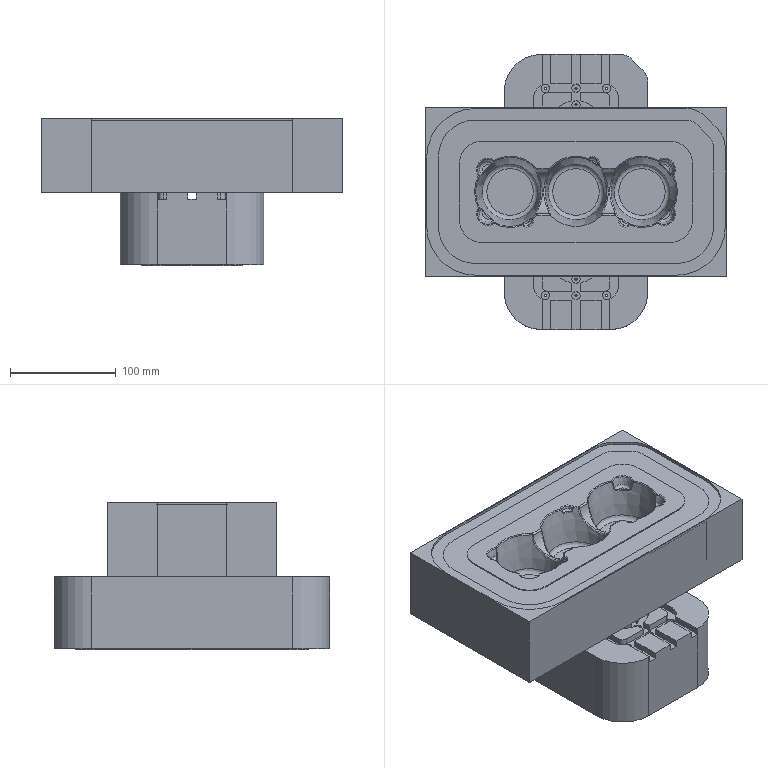NC program | NX | posted with a generic post | part box 284.317 x 260.317 x 139.5 mm
Lines 1 to 931 of 226982:
N10 G17 G21 G94 G90
(B1 , TOOL : D16R0.8)
N12 T00 M6
N14 G53
N16 G17 G0 G90 X-27.032 Y70.7 S7000 M3 M8
N18 G43 Z220.5 H0
N20 Z71.5
N22 G94 G1 X0. Z70.083 F4500.
N24 X103.946
N26 G2 X116.548 Y65.48 R17.822
N28 G1 X127.761 Y54.267
N30 G2 X132.981 Y41.664 R17.822
N32 G1 Y-32.878
N34 G2 X95.159 Y-70.7 R37.822
N36 G1 X-95.159
N38 G2 X-132.981 Y-32.878 R37.822
N40 G1 Y32.878
N42 G2 X-95.159 Y70.7 R37.822
N44 G1 X0.
N46 Y60.62
N48 X103.946
N50 G2 X109.42 Y58.352 R7.742
N52 G1 X120.634 Y47.139
N54 G2 X122.901 Y41.664 R7.742
N56 G1 Y-32.878
N58 G2 X95.159 Y-60.62 R27.742
N60 G1 X-95.159
N62 G2 X-122.901 Y-32.878 R27.742
N64 G1 Y32.878
N66 G2 X-95.159 Y60.62 R27.742
N68 G1 X0.
N70 Y50.54
N72 X102.977
N74 X112.821 Y40.696
N76 Y-32.878
N78 G2 X95.159 Y-50.54 R17.662
N80 G1 X-95.159
N82 G2 X-112.821 Y-32.878 R17.662
N84 G1 Y32.878
N86 G2 X-95.159 Y50.54 R17.662
N88 G1 X0.
N90 Y40.46
N92 X98.802
N94 X102.741 Y36.521
N96 Y-32.878
N98 G2 X95.159 Y-40.46 R7.582
N100 G1 X-95.159
N102 G2 X-102.741 Y-32.878 R7.582
N104 G1 Y32.878
N106 G2 X-95.159 Y40.46 R7.582
N108 G1 X0.
N110 Y30.38
N112 X92.661
N114 Y-30.38
N116 X-92.661
N118 Y30.38
N120 X0.
N122 Y20.3
N124 X82.581
N126 Y-20.3
N128 X-82.581
N130 Y20.3
N132 X0.
N134 Y10.22
N136 X72.501
N138 Y-10.22
N140 X-72.501
N142 Y10.22
N144 X0.
N146 Y0.14
N148 X62.421
N150 Y-0.14
N152 X-62.421
N154 Y0.14
N156 X0.
N158 G3 X3.2 Y3.34 R3.2
N160 G1 Z71.083
N162 G0 Z73.5
N164 X-27.032 Y70.628
N166 Z71.083
N168 G1 X0. Z69.667
N170 X103.946
N172 G2 X116.497 Y65.429 R17.75
N174 G1 X127.71 Y54.215
N176 G2 X132.909 Y41.664 R17.75
N178 G1 Y-32.878
N180 G2 X95.159 Y-70.628 R37.75
N182 G1 X-95.159
N184 G2 X-132.909 Y-32.878 R37.75
N186 G1 Y32.878
N188 G2 X-95.159 Y70.628 R37.75
N190 G1 X0.
N192 Y60.548
N194 X103.946
N196 G2 X109.369 Y58.301 R7.67
N198 G1 X120.582 Y47.088
N200 G2 X122.829 Y41.664 R7.67
N202 G1 Y-32.878
N204 G2 X95.159 Y-60.548 R27.67
N206 G1 X-95.159
N208 G2 X-122.829 Y-32.878 R27.67
N210 G1 Y32.878
N212 G2 X-95.159 Y60.548 R27.67
N214 G1 X0.
N216 Y50.468
N218 X102.947
N220 X112.749 Y40.666
N222 Y-32.878
N224 G2 X95.159 Y-50.468 R17.59
N226 G1 X-95.159
N228 G2 X-112.749 Y-32.878 R17.59
N230 G1 Y32.878
N232 G2 X-95.159 Y50.468 R17.59
N234 G1 X0.
N236 Y40.388
N238 X98.772
N240 X102.669 Y36.491
N242 Y-32.878
N244 G2 X95.159 Y-40.388 R7.51
N246 G1 X-95.159
N248 G2 X-102.669 Y-32.878 R7.51
N250 G1 Y32.878
N252 G2 X-95.159 Y40.388 R7.51
N254 G1 X0.
N256 Y30.308
N258 X92.589
N260 Y-30.308
N262 X-92.589
N264 Y30.308
N266 X0.
N268 Y20.228
N270 X82.509
N272 Y-20.228
N274 X-82.509
N276 Y20.228
N278 X0.
N280 Y10.148
N282 X72.429
N284 Y-10.148
N286 X-72.429
N288 Y10.148
N290 X0.
N292 Y0.068
N294 X62.349
N296 Y-0.068
N298 X-62.349
N300 Y0.068
N302 X0.
N304 G3 X3.2 Y3.268 R3.2
N306 G1 Z70.667
N308 G0 Z73.083
N310 X-27.032 Y70.628
N312 Z70.667
N314 G1 X0. Z69.25
N316 X103.946
N318 G2 X116.497 Y65.429 R17.75
N320 G1 X127.71 Y54.215
N322 G2 X132.909 Y41.664 R17.75
N324 G1 Y-32.878
N326 G2 X95.159 Y-70.628 R37.75
N328 G1 X-95.159
N330 G2 X-132.909 Y-32.878 R37.75
N332 G1 Y32.878
N334 G2 X-95.159 Y70.628 R37.75
N336 G1 X0.
N338 Y60.548
N340 X103.946
N342 G2 X109.369 Y58.301 R7.67
N344 G1 X120.582 Y47.088
N346 G2 X122.829 Y41.664 R7.67
N348 G1 Y-32.878
N350 G2 X95.159 Y-60.548 R27.67
N352 G1 X-95.159
N354 G2 X-122.829 Y-32.878 R27.67
N356 G1 Y32.878
N358 G2 X-95.159 Y60.548 R27.67
N360 G1 X0.
N362 Y50.468
N364 X102.947
N366 X112.749 Y40.666
N368 Y-32.878
N370 G2 X95.159 Y-50.468 R17.59
N372 G1 X-95.159
N374 G2 X-112.749 Y-32.878 R17.59
N376 G1 Y32.878
N378 G2 X-95.159 Y50.468 R17.59
N380 G1 X0.
N382 Y40.388
N384 X98.772
N386 X102.669 Y36.491
N388 Y-32.878
N390 G2 X95.159 Y-40.388 R7.51
N392 G1 X-95.159
N394 G2 X-102.669 Y-32.878 R7.51
N396 G1 Y32.878
N398 G2 X-95.159 Y40.388 R7.51
N400 G1 X0.
N402 Y30.308
N404 X92.589
N406 Y-30.308
N408 X-92.589
N410 Y30.308
N412 X0.
N414 Y20.228
N416 X82.509
N418 Y-20.228
N420 X-82.509
N422 Y20.228
N424 X0.
N426 Y10.148
N428 X72.429
N430 Y-10.148
N432 X-72.429
N434 Y10.148
N436 X0.
N438 Y0.068
N440 X62.349
N442 Y-0.068
N444 X-62.349
N446 Y0.068
N448 X0.
N450 G3 X3.2 Y3.268 R3.2
N452 G1 Z70.25
N454 G0 Z72.667
N456 X-25.442 Y70.628
N458 Z70.25
N460 G1 X0. Z68.917
N462 X103.946
N464 G2 X116.497 Y65.429 R17.75
N466 G1 X127.71 Y54.215
N468 G2 X132.909 Y41.664 R17.75
N470 G1 Y-32.878
N472 G2 X95.159 Y-70.628 R37.75
N474 G1 X-95.159
N476 G2 X-132.909 Y-32.878 R37.75
N478 G1 Y32.878
N480 G2 X-95.159 Y70.628 R37.75
N482 G1 X0.
N484 Y60.548
N486 X103.946
N488 G2 X109.369 Y58.301 R7.67
N490 G1 X120.582 Y47.088
N492 G2 X122.829 Y41.664 R7.67
N494 G1 Y-32.878
N496 G2 X95.159 Y-60.548 R27.67
N498 G1 X-95.159
N500 G2 X-122.829 Y-32.878 R27.67
N502 G1 Y32.878
N504 G2 X-95.159 Y60.548 R27.67
N506 G1 X0.
N508 Y55.845
N510 X89.187
N512 G2 X118.126 Y26.938 R28.939
N514 G1 Y26.847
N516 Y-26.847
N518 Y-26.908
N520 G2 X89.187 Y-55.845 R28.939
N522 G1 X-89.187
N524 G2 X-118.126 Y-26.938 R28.939
N526 G1 Y-26.847
N528 Y26.847
N530 Y26.909
N532 G2 X-89.187 Y55.845 R28.939
N534 G1 X0.
N536 G3 X3.2 Y59.045 R3.2
N538 G1 Z69.917
N540 G0 Z72.25
N542 X-25.442 Y70.628
N544 Z69.917
N546 G1 X0. Z68.583
N548 X103.946
N550 G2 X116.497 Y65.429 R17.75
N552 G1 X127.71 Y54.215
N554 G2 X132.909 Y41.664 R17.75
N556 G1 Y-32.878
N558 G2 X95.159 Y-70.628 R37.75
N560 G1 X-95.159
N562 G2 X-132.909 Y-32.878 R37.75
N564 G1 Y32.878
N566 G2 X-95.159 Y70.628 R37.75
N568 G1 X0.
N570 Y60.548
N572 X103.946
N574 G2 X109.369 Y58.301 R7.67
N576 G1 X120.582 Y47.088
N578 G2 X122.829 Y41.664 R7.67
N580 G1 Y-32.878
N582 G2 X95.159 Y-60.548 R27.67
N584 G1 X-95.159
N586 G2 X-122.829 Y-32.878 R27.67
N588 G1 Y32.878
N590 G2 X-95.159 Y60.548 R27.67
N592 G1 X0.
N594 Y56.055
N596 X89.187
N598 G2 X118.336 Y26.906 R29.15
N600 G1 Y-26.906
N602 G2 X89.187 Y-56.055 R29.15
N604 G1 X-89.187
N606 G2 X-118.336 Y-26.906 R29.15
N608 G1 Y26.906
N610 G2 X-89.187 Y56.055 R29.15
N612 G1 X0.
N614 G3 X3.2 Y59.255 R3.2
N616 G1 Z69.583
N618 G0 Z71.917
N620 X-25.442 Y70.628
N622 Z69.583
N624 G1 X0. Z68.25
N626 X103.946
N628 G2 X116.497 Y65.429 R17.75
N630 G1 X127.71 Y54.215
N632 G2 X132.909 Y41.664 R17.75
N634 G1 Y-32.878
N636 G2 X95.159 Y-70.628 R37.75
N638 G1 X-95.159
N640 G2 X-132.909 Y-32.878 R37.75
N642 G1 Y32.878
N644 G2 X-95.159 Y70.628 R37.75
N646 G1 X0.
N648 Y60.548
N650 X103.946
N652 G2 X109.369 Y58.301 R7.67
N654 G1 X120.582 Y47.088
N656 G2 X122.829 Y41.664 R7.67
N658 G1 Y-32.878
N660 G2 X95.159 Y-60.548 R27.67
N662 G1 X-95.159
N664 G2 X-122.829 Y-32.878 R27.67
N666 G1 Y32.878
N668 G2 X-95.159 Y60.548 R27.67
N670 G1 X0.
N672 Y56.126
N674 X89.149
N676 X89.19
N678 G2 X118.407 Y26.938 R29.22
N680 G1 Y26.847
N682 Y-26.847
N684 Y-26.91
N686 G2 X89.229 Y-56.126 R29.22
N688 G1 X89.149
N690 X-89.149
N692 X-89.19
N694 G2 X-118.407 Y-26.938 R29.22
N696 G1 Y-26.847
N698 Y26.847
N700 Y26.91
N702 G2 X-89.229 Y56.126 R29.22
N704 G1 X-89.149
N706 X0.
N708 G3 X3.2 Y59.326 R3.2
N710 G1 Z69.25
N712 G0 Z72.25
N714 X-1.969 Y25.197
N716 Z70.25
N718 G1 X0.477 Y25.318 Z70.122
N720 X3.927 Y25.016 Z69.94
N722 X7.303 Y24.246 Z69.759
N724 X8.465 Y23.834 Z69.694
N726 X9.124 Y23.607 Z69.658
N728 X10.449 Y23.388 Z69.587
N730 X11.791 Y23.391 Z69.517
N732 X13.115 Y23.614 Z69.446
N734 X13.773 Y23.844 Z69.41
N736 X13.899 Y23.163 Z69.374
N738 X14.363 Y21.903 Z69.303
N740 X15.031 Y20.738 Z69.233
N742 X15.884 Y19.701 Z69.162
N744 X16.408 Y19.248 Z69.126
N746 X17.346 Y18.448 Z69.062
N748 X18.207 Y17.599 Z68.998
N750 X19.019 Y16.673 Z68.934
N752 X19.125 Y16.55 Z68.925
N754 X19.236 Y16.432 Z68.917
N756 G3 X25.473 Y13.698 R8.607
N758 G1 X36.894
N760 G3 X43.347 Y16.673 R8.606
N762 G2 X73.834 Y22.543 R25.293
N764 G3 X82.098 Y23.018 R8.217
N766 G2 X85.384 Y19.732 R2.371
N768 G3 X84.909 Y11.468 R8.217
N770 G2 X84.909 Y-11.468 R25.293
N772 G3 X85.384 Y-19.732 R8.217
N774 G2 X82.098 Y-23.018 R2.371
N776 G3 X73.834 Y-22.543 R8.217
N778 G2 X53.901 Y-23.834 R25.293
N780 G3 X48.604 Y-23.835 R8.119
N782 X45.957 Y-19.248 R8.211
N784 G2 X43.347 Y-16.673 R25.293
N786 G3 X36.893 Y-13.698 R9.004
N788 G1 X24.765
N790 G3 X18.258 Y-16.812 R8.934
N792 G1 X18.22 Y-16.84
N794 G2 X-18.22 Y-16.84 R24.81
N796 G1 X-18.258 Y-16.812
N798 G3 X-24.765 Y-13.698 R8.934
N800 G1 X-36.894
N802 G3 X-43.347 Y-16.673 R8.606
N804 G2 X-45.957 Y-19.248 R25.293
N806 G3 X-48.602 Y-23.84 R8.184
N808 X-53.901 Y-23.834 R8.043
N810 G2 X-73.834 Y-22.543 R25.293
N812 G3 X-82.098 Y-23.018 R8.217
N814 G2 X-85.384 Y-19.732 R2.371
N816 G3 X-84.909 Y-11.468 R8.217
N818 G2 X-84.909 Y11.468 R25.293
N820 G3 X-85.384 Y19.732 R8.217
N822 G2 X-82.098 Y23.018 R2.371
N824 G3 X-73.834 Y22.543 R8.217
N826 G2 X-43.347 Y16.673 R25.293
N828 G3 X-36.893 Y13.698 R9.004
N830 G1 X-25.472
N832 G3 X-19.019 Y16.673 R8.606
N834 G2 X8.465 Y23.834 R25.293
N836 G3 X13.773 Y23.844 R8.097
N838 X16.408 Y19.248 R7.989
N840 G2 X19.019 Y16.673 R25.293
N842 G3 X19.236 Y16.432 R8.607
N844 G1 X11.867 Y9.554
N846 G3 X25.441 Y3.618 R18.687
N848 G1 X36.926
N850 G3 X50.941 Y10.045 R18.686
N852 G2 X69.263 Y13.559 R15.213
N854 G3 X74.24 Y11.874 R18.297
N856 X75.925 Y6.898 R18.297
N858 G2 X75.925 Y-6.897 R15.213
N860 G3 X74.24 Y-11.874 R18.297
N862 X69.264 Y-13.559 R18.297
N864 G2 X57.231 Y-14.32 R15.213
N866 G3 X54.505 Y-13.603 R18.199
N868 X52.547 Y-11.62 R18.291
N870 G2 X50.881 Y-9.976 R15.213
N872 G3 X48.651 Y-7.855 R19.084
N874 G1 X54.987 Y-0.015
N876 G3 X58.523 Y3.402 R28.766
N878 G2 X64.693 Y4.575 R5.133
N880 G3 X66.22 Y3.854 R28.377
N882 X66.94 Y2.328 R28.377
N884 G2 X66.941 Y-2.327 R5.133
N886 G3 X66.22 Y-3.854 R28.377
N888 X64.694 Y-4.574 R28.377
N890 G2 X60.588 Y-4.815 R5.133
N892 G3 X59.745 Y-4.535 R28.279
N894 X59.107 Y-3.966 R28.371
N896 G2 X58.443 Y-3.311 R5.133
N898 G3 X54.987 Y-0.015 R29.164
N900 G1 X48.651 Y-7.855
N902 G3 X37.025 Y-3.618 R19.084
N904 G1 X24.61
N906 G3 X11.547 Y-9.232 R19.014
N908 G1 X11.483 Y-9.278
N910 X10.817 Y-9.998
N912 G2 X-10.817 Y-9.998 R14.73
N914 G1 X-11.485 Y-9.276
N916 X-11.548 Y-9.23
N918 G3 X-24.61 Y-3.618 R19.014
N920 G1 X-36.926
N922 G3 X-50.941 Y-10.044 R18.686
N924 G2 X-52.545 Y-11.618 R15.213
N926 G3 X-54.504 Y-13.601 R18.264
N928 X-57.244 Y-14.324 R18.123
N930 G2 X-69.263 Y-13.559 R15.213
N932 G3 X-74.24 Y-11.874 R18.297
N934 X-75.925 Y-6.898 R18.297
N936 G2 X-75.925 Y6.897 R15.213
N938 G3 X-74.24 Y11.874 R18.297
N940 X-69.264 Y13.559 R18.297
N942 G2 X-50.881 Y9.976 R15.213
N944 G3 X-48.651 Y7.855 R19.084
N946 G1 X-54.987 Y0.015
N948 G3 X-58.523 Y-3.403 R28.766
N950 G2 X-59.053 Y-3.92 R5.133
N952 G1 X-59.155 Y-4.008
N954 G3 X-59.745 Y-4.534 R28.344
N956 X-60.605 Y-4.821 R28.203
N958 G2 X-64.693 Y-4.575 R5.133
N960 G3 X-66.22 Y-3.854 R28.377
N962 X-66.94 Y-2.328 R28.377
N964 G2 X-66.941 Y2.327 R5.133
N966 G3 X-66.22 Y3.854 R28.377
N968 X-64.694 Y4.574 R28.377
N970 G2 X-58.443 Y3.311 R5.133
N972 G3 X-54.987 Y0.015 R29.164
N974 G1 X-48.651 Y7.855
N976 G3 X-37.025 Y3.618 R19.084
N978 G1 X-25.44
N980 G3 X-11.425 Y10.045 R18.686
N982 G2 X5.135 Y14.32 R15.213
N984 G3 X7.851 Y13.605 R18.177
N986 X9.845 Y11.597 R18.069
N988 G2 X11.425 Y10.044 R15.213
N990 G3 X11.867 Y9.554 R18.687
N992 G1 X4.498 Y2.676
N994 G3 X7.062 Y0.247 R28.767
N996 X5.026 Y-1.512 R29.094
N998 G1 X4.747 Y-1.715
N1000 X3.415 Y-3.156
N1002 G2 X-3.415 Y-3.156 R4.65
N1004 G1 X-4.75 Y-1.712
N1006 X-5.029 Y-1.509
N1008 G3 X-7.062 Y0.247 R29.094
N1010 X-3.843 Y3.402 R28.766
N1012 G2 X1.779 Y4.815 R5.133
N1014 G3 X2.617 Y4.536 R28.257
N1016 X3.296 Y3.934 R28.149
N1018 G2 X3.843 Y3.402 R5.133
N1020 G3 X4.498 Y2.676 R28.767
N1022 X9.021 Y2.52 R3.2
N1024 G1 Z69.917
N1026 G0 Z72.25
N1028 X-2.547 Y24.779
N1030 Z69.917
N1032 G1 X0.509 Y24.926 Z69.756
N1034 X3.91 Y24.623 Z69.577
N1036 X7.238 Y23.857 Z69.398
N1038 X8.389 Y23.445 Z69.334
N1040 X9.057 Y23.212 Z69.297
N1042 X10.912 Y22.951 Z69.199
N1044 X12.779 Y23.111 Z69.101
N1046 X13.458 Y23.308 Z69.064
N1048 X13.629 Y22.619 Z69.027
N1050 X14.424 Y20.928 Z68.929
N1052 X15.572 Y19.453 Z68.831
N1054 X16.109 Y18.988 Z68.793
N1056 X17.042 Y18.197 Z68.729
N1058 X17.919 Y17.334 Z68.665
N1060 X18.725 Y16.415 Z68.601
N1062 X18.834 Y16.288 Z68.592
N1064 X18.947 Y16.165 Z68.583
N1066 G3 X25.541 Y13.241 R9.107
N1068 G1 X36.825
N1070 G3 X43.641 Y16.415 R9.107
N1072 G2 X73.67 Y22.188 R24.901
N1074 G3 X82.311 Y22.69 R8.573
N1076 G2 X85.056 Y19.945 R1.979
N1078 G3 X84.554 Y11.304 R8.717
N1080 G2 X84.554 Y-11.304 R24.901
N1082 G3 X85.056 Y-19.945 R8.691
N1084 G2 X82.311 Y-22.69 R1.979
N1086 G3 X73.67 Y-22.188 R8.685
N1088 G2 X53.976 Y-23.445 R24.901
N1090 G3 X48.918 Y-23.32 R8.134
N1092 X46.256 Y-18.988 R8.489
N1094 G2 X43.641 Y-16.415 R24.901
N1096 G3 X36.825 Y-13.241 R9.107
N1098 G1 X24.966
N1100 G3 X18.558 Y-16.173 R8.954
N1102 G1 X18.103 Y-16.683
N1104 X18.058 Y-16.705
N1106 G2 X-18.058 Y-16.706 R24.6
N1108 G1 X-18.102 Y-16.683
N1110 X-18.558 Y-16.173
N1112 G3 X-24.967 Y-13.241 R8.998
N1114 G1 X-36.825
N1116 G3 X-43.641 Y-16.415 R9.107
N1118 G2 X-46.257 Y-18.988 R24.901
N1120 G3 X-48.913 Y-23.301 R8.385
N1122 X-53.976 Y-23.445 R8.465
N1124 G2 X-73.67 Y-22.188 R24.901
N1126 G3 X-82.311 Y-22.69 R8.572
N1128 G2 X-85.056 Y-19.945 R1.979
N1130 G3 X-84.554 Y-11.304 R8.717
N1132 G2 X-84.554 Y11.304 R24.901
N1134 G3 X-85.056 Y19.945 R8.686
N1136 G2 X-82.311 Y22.69 R1.979
N1138 G3 X-73.67 Y22.188 R8.685
N1140 G2 X-43.641 Y16.415 R24.901
N1142 G3 X-36.825 Y13.241 R9.106
N1144 G1 X-25.541
N1146 G3 X-18.725 Y16.415 R9.106
N1148 G2 X8.389 Y23.445 R24.901
N1150 G3 X13.458 Y23.308 R8.316
N1152 X16.109 Y18.988 R8.397
N1154 G2 X18.725 Y16.415 R24.901
N1156 G3 X18.947 Y16.165 R9.107
N1158 G1 X11.545 Y9.323
N1160 G3 X25.489 Y3.161 R19.187
N1162 G1 X36.877
N1164 G3 X51.244 Y9.797 R19.187
N1166 G2 X69.094 Y13.206 R14.821
N1168 G3 X73.92 Y11.532 R18.653
N1170 X75.55 Y6.772 R18.797
N1172 G2 X75.554 Y-6.764 R14.821
N1174 G3 X73.914 Y-11.547 R18.771
N1176 X69.128 Y-13.189 R18.765
N1178 G2 X57.36 Y-13.95 R14.821
N1180 G3 X54.715 Y-13.228 R18.214
N1182 X52.824 Y-11.341 R18.569
N1184 G2 X51.244 Y-9.797 R14.821
N1186 G3 X49.121 Y-7.697 R19.187
N1188 G1 X55.63 Y0.
N1190 G3 X58.828 Y3.156 R29.267
N1192 G2 X64.518 Y4.224 R4.741
N1194 G3 X65.928 Y3.554 R28.733
N1196 X66.559 Y2.213 R28.877
N1198 G2 X66.565 Y-2.202 R4.741
N1200 G3 X65.925 Y-3.559 R28.851
N1202 X64.566 Y-4.2 R28.845
N1204 G2 X60.751 Y-4.458 R4.741
N1206 G3 X59.945 Y-4.184 R28.294
N1208 X59.364 Y-3.671 R28.649
N1210 G2 X58.828 Y-3.156 R4.741
N1212 G3 X55.63 Y0. R29.267
N1214 G1 X49.121 Y-7.697
N1216 G3 X36.877 Y-3.161 R19.187
N1218 G1 X24.842
N1220 G3 X10.952 Y-9.556 R19.034
N1222 X10.659 Y-9.86 R10.08
N1224 G2 X-10.659 Y-9.861 R14.52
N1226 G3 X-10.952 Y-9.557 R10.08
N1228 X-24.833 Y-3.161 R19.078
N1230 G1 X-36.877
N1232 G3 X-51.244 Y-9.797 R19.187
N1234 G2 X-52.81 Y-11.329 R14.821
N1236 G3 X-54.728 Y-13.238 R18.465
N1238 X-57.319 Y-13.935 R18.545
N1240 G2 X-69.094 Y-13.206 R14.821
N1242 G3 X-73.92 Y-11.532 R18.652
N1244 X-75.55 Y-6.772 R18.797
N1246 G2 X-75.554 Y6.763 R14.821
N1248 G3 X-73.913 Y11.547 R18.766
N1250 X-69.128 Y13.189 R18.765
N1252 G2 X-51.245 Y9.797 R14.821
N1254 G3 X-49.121 Y7.697 R19.186
N1256 G1 X-55.63 Y0.
N1258 G3 X-58.828 Y-3.156 R29.267
N1260 G2 X-59.344 Y-3.653 R4.741
N1262 G3 X-59.95 Y-4.187 R28.545
N1264 X-60.694 Y-4.437 R28.625
N1266 G2 X-64.518 Y-4.225 R4.741
N1268 G3 X-65.928 Y-3.554 R28.732
N1270 X-66.559 Y-2.213 R28.877
N1272 G2 X-66.566 Y2.2 R4.741
N1274 G3 X-65.925 Y3.559 R28.846
N1276 X-64.566 Y4.2 R28.845
N1278 G2 X-58.828 Y3.156 R4.741
N1280 G3 X-55.63 Y0. R29.266
N1282 G1 X-49.121 Y7.697
N1284 G3 X-36.877 Y3.161 R19.186
N1286 G1 X-25.489
N1288 G3 X-11.121 Y9.797 R19.186
N1290 G2 X5.026 Y13.943 R14.821
N1292 G3 X7.645 Y13.233 R18.396
N1294 X9.55 Y11.335 R18.477
N1296 G2 X11.121 Y9.797 R14.821
N1298 G3 X11.545 Y9.323 R19.187
N1300 G1 X4.143 Y2.481
N1302 G3 X6.54 Y0.167 R29.267
N1304 X3.61 Y-2.646 R29.114
N1306 X3.259 Y-3.015 R20.16
N1308 G2 X-3.259 Y-3.015 R4.44
N1310 G3 X-3.613 Y-2.643 R20.16
N1312 X-6.542 Y0.165 R29.158
N1314 X-3.538 Y3.156 R29.266
N1316 G2 X1.642 Y4.448 R4.741
N1318 G3 X2.418 Y4.186 R28.476
N1320 X3.013 Y3.661 R28.557
N1322 G2 X3.538 Y3.156 R4.741
N1324 G3 X4.143 Y2.481 R29.267
N1326 X8.665 Y2.303 R3.2
N1328 G1 Z69.583
N1330 G0 Z71.917
N1332 X-2.856 Y24.523
N1334 Z69.583
N1336 G1 X-2.852
N1338 X0.529 Y24.683 Z69.406
N1340 X3.9 Y24.379 Z69.228
N1342 X7.198 Y23.616 Z69.051
N1344 X8.343 Y23.205 Z68.987
N1346 X9.017 Y22.968 Z68.95
N1348 X10.796 Y22.704 Z68.855
N1350 X12.591 Y22.819 Z68.761
N1352 X13.283 Y22.998 Z68.724
N1354 X13.465 Y22.316 Z68.687
N1356 X14.26 Y20.695 Z68.592
N1358 X15.386 Y19.284 Z68.498
N1360 X15.924 Y18.827 Z68.461
N1362 X16.853 Y18.042 Z68.397
N1364 X17.741 Y17.17 Z68.332
N1366 X18.543 Y16.255 Z68.268
N1368 X18.654 Y16.126 Z68.259
N1370 X18.77 Y16.001 Z68.25
N1372 G3 X25.602 Y12.942 R9.551
N1374 G1 X36.764
N1376 G3 X42.976 Y15.406 R9.293
N1378 X43.823 Y16.255 R34.483
N1380 G2 X73.568 Y21.967 R24.659
N1382 G3 X82.444 Y22.487 R8.893
N1384 G2 X84.853 Y20.078 R1.737
N1386 G3 X84.333 Y11.202 R8.9
N1388 G2 X84.333 Y-11.202 R24.659
N1390 G3 X84.853 Y-20.078 R8.898
N1392 G2 X82.444 Y-22.487 R1.737
N1394 G3 X73.568 Y-21.967 R8.893
N1396 G2 X54.023 Y-23.205 R24.659
N1398 G3 X49.095 Y-22.989 R8.543
N1400 X46.442 Y-18.827 R8.496
N1402 G2 X43.823 Y-16.255 R24.659
N1404 G3 X42.976 Y-15.406 R34.484
N1406 X36.764 Y-12.942 R9.275
N1408 G1 X25.146
N1410 G3 X18.9 Y-15.667 R8.739
N1412 G1 X18.558 Y-16.043
N1414 X18.438 Y-16.166
N1416 G2 X-18.441 Y-16.162 R24.522
N1418 G3 X-25.146 Y-12.942 R8.856
N1420 G1 X-36.764
N1422 G3 X-43.823 Y-16.255 R9.563
N1424 G2 X-46.442 Y-18.827 R24.659
N1426 G3 X-49.09 Y-22.989 R8.412
N1428 X-54.023 Y-23.205 R8.534
N1430 G2 X-73.568 Y-21.967 R24.659
N1432 G3 X-82.444 Y-22.487 R8.893
N1434 G2 X-84.853 Y-20.078 R1.737
N1436 G3 X-84.333 Y-11.202 R8.898
N1438 G2 X-84.333 Y11.202 R24.659
N1440 G3 X-84.853 Y20.078 R8.9
N1442 G2 X-82.444 Y22.487 R1.737
N1444 G3 X-73.568 Y21.967 R8.893
N1446 G2 X-43.823 Y16.255 R24.659
N1448 G3 X-36.764 Y12.942 R9.563
N1450 G1 X-25.602
N1452 G3 X-18.543 Y16.255 R9.471
N1454 G2 X8.343 Y23.205 R24.659
N1456 G3 X13.283 Y22.998 R8.487
N1458 X15.924 Y18.827 R8.283
N1460 G2 X18.543 Y16.255 R24.659
N1462 G3 X18.77 Y16.001 R9.551
N1464 G1 X11.374 Y9.151
N1466 G3 X25.509 Y2.862 R19.631
N1468 G1 X36.815
N1470 G3 X49.898 Y8.079 R19.373
N1472 X51.077 Y9.256 R44.563
N1474 G1 X51.244 Y9.429
N1476 G2 X69.019 Y12.972 R14.579
N1478 G3 X73.705 Y11.338 R18.973
N1480 X75.337 Y6.655 R18.98
N1482 G2 X75.338 Y-6.654 R14.579
N1484 G3 X73.705 Y-11.338 R18.978
N1486 X69.019 Y-12.972 R18.973
N1488 G2 X57.393 Y-13.704 R14.579
N1490 G3 X54.859 Y-13.008 R18.623
N1492 X52.976 Y-11.152 R18.576
N1494 G2 X51.403 Y-9.61 R14.579
N1496 G1 X51.244 Y-9.429
N1498 X51.077 Y-9.256
N1500 G3 X49.901 Y-8.081 R44.564
N1502 X49.376 Y-7.608 R19.355
N1504 G1 X55.989 Y0.
N1506 G3 X56.834 Y0.763 R29.453
N1508 X58.332 Y2.257 R54.643
N1510 G1 X58.723 Y2.663
N1512 X58.933 Y2.91
N1514 G2 X64.45 Y3.987 R4.499
N1516 G3 X65.74 Y3.374 R29.053
N1518 X66.351 Y2.088 R29.06
N1520 G2 X66.352 Y-2.087 R4.499
N1522 G3 X65.74 Y-3.374 R29.058
N1524 X64.451 Y-3.987 R29.053
N1526 G2 X60.788 Y-4.213 R4.499
N1528 G3 X60.074 Y-3.971 R28.703
N1530 X59.495 Y-3.464 R28.656
N1532 G2 X58.983 Y-2.966 R4.499
N1534 G1 X58.332 Y-2.257
N1536 G3 X56.839 Y-0.768 R54.644
N1538 X55.989 Y0. R29.435
N1540 G1 X49.376 Y-7.608
N1542 G3 X36.811 Y-2.862 R19.355
N1544 G1 X25.091
N1546 G3 X11.214 Y-9.136 R18.819
N1548 G1 X11.027 Y-9.329
N1550 G2 X-10.792 Y-9.597 R14.442
N1552 G3 X-25.074 Y-2.862 R18.936
N1554 G1 X-36.86
N1556 G3 X-51.421 Y-9.63 R19.643
N1558 G2 X-52.968 Y-11.145 R14.579
N1560 G3 X-54.862 Y-13.008 R18.492
N1562 X-57.395 Y-13.705 R18.614
N1564 G2 X-69.019 Y-12.972 R14.579
N1566 G3 X-73.705 Y-11.338 R18.973
N1568 X-75.338 Y-6.654 R18.978
N1570 G2 X-75.337 Y6.655 R14.579
N1572 G3 X-73.705 Y11.338 R18.98
N1574 X-69.019 Y12.972 R18.973
N1576 G2 X-51.421 Y9.63 R14.579
N1578 G3 X-49.417 Y7.631 R19.643
N1580 G1 X-56.002 Y0.
N1582 G3 X-59.003 Y-2.988 R29.723
N1584 G2 X-59.466 Y-3.439 R4.499
N1586 G3 X-60.075 Y-3.971 R28.572
N1588 X-60.791 Y-4.214 R28.694
N1590 G2 X-64.451 Y-3.987 R4.499
N1592 G3 X-65.74 Y-3.374 R29.053
N1594 X-66.352 Y-2.087 R29.058
N1596 G2 X-66.351 Y2.088 R4.499
N1598 G3 X-65.74 Y3.374 R29.06
N1600 X-64.451 Y3.987 R29.053
N1602 G2 X-59.003 Y2.988 R4.499
N1604 G3 X-56.002 Y0. R29.723
N1606 G1 X-49.417 Y7.631
N1608 G3 X-36.86 Y2.862 R19.643
N1610 G1 X-25.528
N1612 G3 X-10.935 Y9.642 R19.551
N1614 G2 X4.969 Y13.706 R14.579
N1616 G3 X7.501 Y13.009 R18.567
N1618 X9.409 Y11.136 R18.363
N1620 G2 X10.944 Y9.632 R14.579
N1622 G3 X11.374 Y9.151 R19.631
N1624 G1 X3.979 Y2.302
N1626 G3 X6.248 Y0.099 R29.711
N1628 X3.853 Y-2.248 R28.899
N1630 G1 X3.554 Y-2.556
N1632 X3.331 Y-2.819
N1634 G2 X-3.203 Y-2.961 R4.362
N1636 G3 X-6.238 Y0.102 R29.016
N1638 X-3.352 Y3.001 R29.631
N1640 G2 X1.573 Y4.215 R4.499
N1642 G3 X2.289 Y3.971 R28.647
N1644 X2.897 Y3.442 R28.443
N1646 G2 X3.361 Y2.99 R4.499
N1648 G3 X3.979 Y2.302 R29.711
N1650 X8.501 Y2.129 R3.2
N1652 G1 Z69.25
N1654 G0 Z71.583
N1656 X-5.244 Y23.873
N1658 Z69.25
N1660 G1 X-2.81 Y24.325 Z69.12
N1662 X0.545 Y24.481 Z68.944
N1664 X3.891 Y24.176 Z68.768
N1666 X7.164 Y23.416 Z68.592
N1668 X8.303 Y23.004 Z68.529
N1670 X8.98 Y22.763 Z68.491
N1672 X10.693 Y22.489 Z68.4
N1674 X12.425 Y22.564 Z68.309
N1676 X13.126 Y22.725 Z68.271
N1678 X13.335 Y22.038 Z68.234
N1680 X14.134 Y20.503 Z68.143
N1682 X15.224 Y19.159 Z68.052
N1684 X15.771 Y18.693 Z68.015
N1686 X16.697 Y17.912 Z67.951
N1688 X17.592 Y17.033 Z67.886
N1690 X18.391 Y16.122 Z67.822
N1692 X18.63 Y15.869 Z67.804
N1694 X18.821 Y15.667
N1696 G3 X25.684 Y12.663 R9.509
N1698 G1 X36.682
N1700 G3 X40.961 Y13.709 R9.587
N1702 X43.975 Y16.122 R10.73
N1704 G2 X73.484 Y21.784 R24.457
N1706 G3 X82.588 Y22.34 R9.023
N1708 G2 X84.684 Y20.188 R1.535
N1710 G3 X84.15 Y11.118 R9.081
N1712 G2 X84.15 Y-11.118 R24.457
N1714 G3 X84.684 Y-20.188 R9.069
N1716 G2 X82.588 Y-22.34 R1.535
N1718 G3 X73.484 Y-21.784 R9.023
N1720 G2 X54.063 Y-23.004 R24.457
N1722 G3 X49.238 Y-22.741 R8.318
N1724 X46.595 Y-18.693 R8.516
N1726 G2 X43.975 Y-16.122 R24.457
N1728 G1 X43.286 Y-15.422
N1730 G3 X36.693 Y-12.663 R9.257
N1732 G1 X25.393
N1734 G3 X18.558 Y-15.906 R9.086
N1736 G1 X18.378 Y-16.113
N1738 G2 X-18.558 Y-15.906 R24.442
N1740 G3 X-25.393 Y-12.663 R9.1
N1742 G1 X-36.682
N1744 G3 X-40.961 Y-13.709 R9.634
N1746 X-43.975 Y-16.122 R10.602
N1748 G2 X-46.595 Y-18.693 R24.457
N1750 G3 X-49.235 Y-22.735 R8.459
N1752 X-54.063 Y-23.004 R8.425
N1754 G2 X-73.483 Y-21.784 R24.457
N1756 G3 X-82.588 Y-22.34 R9.023
N1758 G2 X-84.684 Y-20.188 R1.535
N1760 G3 X-84.15 Y-11.118 R9.069
N1762 G2 X-84.15 Y11.118 R24.457
N1764 G3 X-84.684 Y20.188 R9.069
N1766 G2 X-82.588 Y22.34 R1.535
N1768 G3 X-73.483 Y21.784 R9.023
N1770 G2 X-43.975 Y16.122 R24.457
N1772 G1 X-43.544 Y15.667
N1774 G3 X-36.682 Y12.663 R9.489
N1776 G1 X-25.684
N1778 G3 X-18.822 Y15.667 R9.5
N1780 G1 X-18.474 Y16.057
N1782 X-18.391 Y16.122
N1784 G2 X8.303 Y23.004 R24.457
N1786 G3 X13.126 Y22.725 R8.595
N1788 X15.771 Y18.693 R8.583
N1790 G2 X18.391 Y16.122 R24.457
N1792 G1 X18.63 Y15.869
N1794 X11.308 Y8.942
N1796 X11.486 Y8.753
N1798 G3 X25.645 Y2.583 R19.589
N1800 G1 X36.721
N1802 G3 X45.642 Y4.781 R19.667
N1804 X51.567 Y9.491 R20.81
N1806 G2 X68.915 Y12.799 R14.377
N1808 G3 X73.534 Y11.159 R19.103
N1810 X75.156 Y6.566 R19.161
N1812 G2 X75.158 Y-6.562 R14.377
N1814 G3 X73.533 Y-11.16 R19.149
N1816 X68.915 Y-12.799 R19.103
N1818 G2 X57.494 Y-13.526 R14.377
N1820 G3 X54.961 Y-12.807 R18.398
N1822 X53.11 Y-11.001 R18.596
N1824 G2 X51.555 Y-9.477 R14.377
N1826 G1 X51.361 Y-9.256
N1828 X50.465 Y-8.347
N1830 G3 X49.59 Y-7.513 R19.337
N1832 G1 X56.314 Y-0.003
N1834 G3 X59.148 Y2.848 R30.89
N1836 G2 X64.338 Y3.818 R4.297
N1838 G3 X65.588 Y3.219 R29.183
N1840 X66.172 Y1.995 R29.241
N1842 G2 X66.174 Y-1.991 R4.297
N1844 G3 X65.588 Y-3.22 R29.229
N1846 X64.338 Y-3.818 R29.183
N1848 G2 X60.917 Y-4.045 R4.297
N1850 G3 X60.175 Y-3.788 R28.478
N1852 X59.615 Y-3.301 R28.676
N1854 G2 X59.135 Y-2.833 R4.297
N1856 G1 X57.644 Y-1.271
N1858 G3 X56.314 Y-0.003 R29.417
N1860 G1 X49.59 Y-7.513